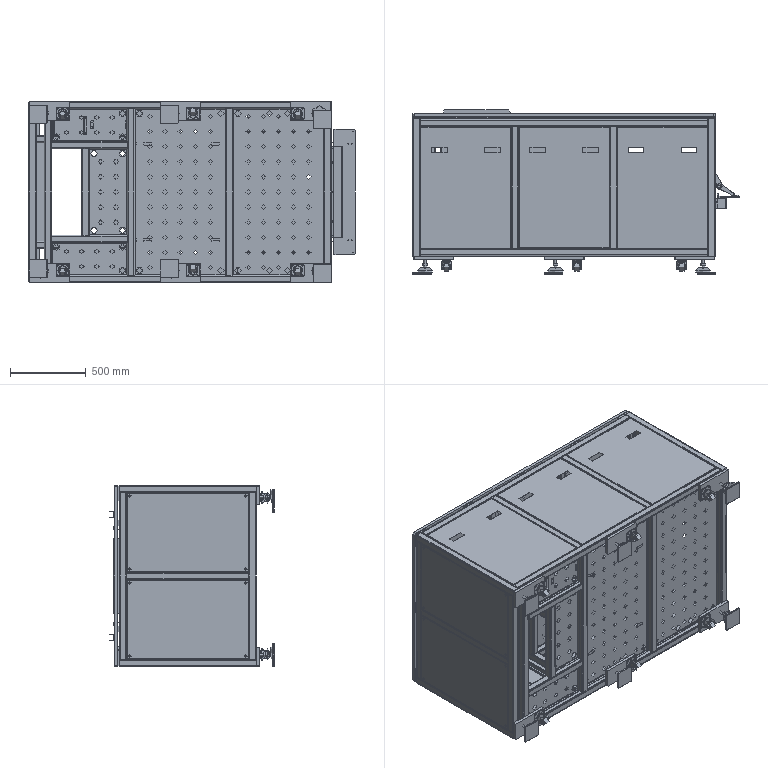Part | NX | 199 solids | 7361 faces | volume 114322472 mm3 | plane 4129 | cylinder 2518 | cone 358 | spline 284 | torus 64 | sphere 8 | commonest cylinder face diameters 4 x218 30 x206 14 x194 5 x176 2 x142 4.2 x118